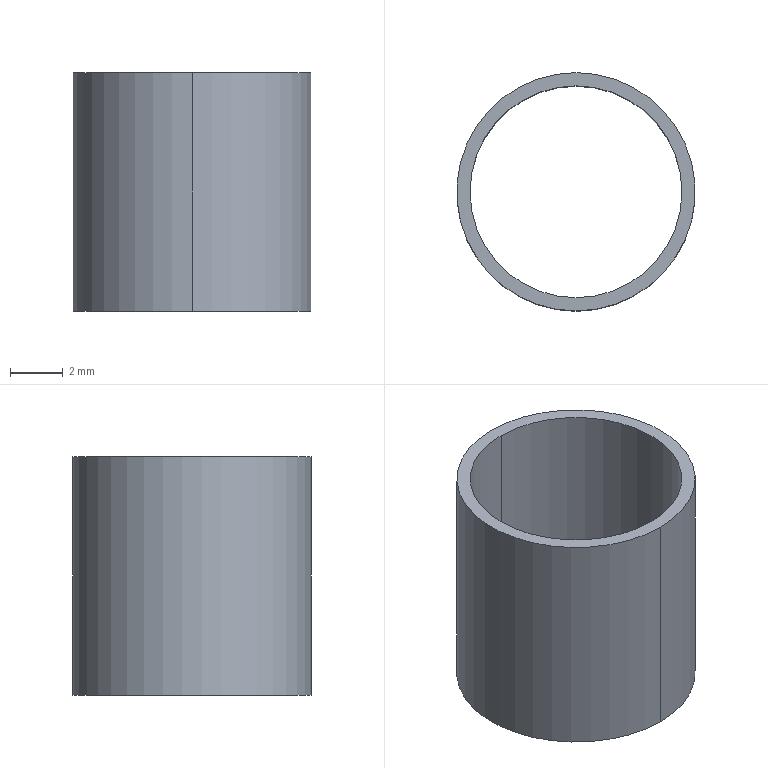Part | STEP file | ASND-0110-4216111700 | 1 solid | 6 faces | box 9 x 9 x 9 mm | volume 120.166 mm3 | cylinder 4 | plane 2 | commonest cylinder face diameters 8 x2 9 x2
STEP:
#1=CARTESIAN_POINT('',(0.,0.,0.));
#2=DIRECTION('',(0.,0.,1.));
#3=DIRECTION('',(1.,0.,0.));
#4=AXIS2_PLACEMENT_3D('',#1,#2,#3);
#5=CARTESIAN_POINT('',(0.,-4.,9.));
#6=VERTEX_POINT('',#5);
#7=CARTESIAN_POINT('',(0.,-4.,0.));
#8=VERTEX_POINT('',#7);
#9=CARTESIAN_POINT('',(0.,-4.,9.45));
#10=DIRECTION('',(0.,0.,-1.));
#11=VECTOR('',#10,1.);
#12=LINE('',#9,#11);
#13=CARTESIAN_POINT('',(0.,0.,9.45));
#14=DIRECTION('',(0.,0.,-1.));
#15=DIRECTION('',(0.,-1.,0.));
#16=AXIS2_PLACEMENT_3D('',#13,#14,#15);
#17=CYLINDRICAL_SURFACE('',#16,4.);
#18=CARTESIAN_POINT('',(6.283,0.));
#19=DIRECTION('',(0.,1.));
#20=VECTOR('',#19,1.);
#21=LINE('',#18,#20);
#22=(GEOMETRIC_REPRESENTATION_CONTEXT(2)PARAMETRIC_REPRESENTATION_CONTEXT()REPRESENTATION_CONTEXT('',''));
#23=DEFINITIONAL_REPRESENTATION('',(#21),#22);
#24=PCURVE('',#17,#23);
#25=CARTESIAN_POINT('',(0.,0.,9.45));
#26=DIRECTION('',(0.,0.,-1.));
#27=DIRECTION('',(0.,-1.,0.));
#28=AXIS2_PLACEMENT_3D('',#25,#26,#27);
#29=CYLINDRICAL_SURFACE('',#28,4.);
#30=CARTESIAN_POINT('',(0.,0.));
#31=DIRECTION('',(0.,1.));
#32=VECTOR('',#31,1.);
#33=LINE('',#30,#32);
#34=(GEOMETRIC_REPRESENTATION_CONTEXT(2)PARAMETRIC_REPRESENTATION_CONTEXT()REPRESENTATION_CONTEXT('',''));
#35=DEFINITIONAL_REPRESENTATION('',(#33),#34);
#36=PCURVE('',#29,#35);
#37=SURFACE_CURVE('',#12,(#24,#36),.PCURVE_S1.);
#38=EDGE_CURVE('',#6,#8,#37,.T.);
#39=ORIENTED_EDGE('',*,*,#38,.T.);
#40=CARTESIAN_POINT('',(0.,4.,0.));
#41=VERTEX_POINT('',#40);
#42=CARTESIAN_POINT('',(0.,0.,0.));
#43=DIRECTION('',(0.,0.,-1.));
#44=DIRECTION('',(0.,1.,0.));
#45=AXIS2_PLACEMENT_3D('',#42,#43,#44);
#46=CIRCLE('',#45,4.);
#47=CARTESIAN_POINT('',(3.142,9.45));
#48=DIRECTION('',(1.,0.));
#49=VECTOR('',#48,1.);
#50=LINE('',#47,#49);
#51=(GEOMETRIC_REPRESENTATION_CONTEXT(2)PARAMETRIC_REPRESENTATION_CONTEXT()REPRESENTATION_CONTEXT('',''));
#52=DEFINITIONAL_REPRESENTATION('',(#50),#51);
#53=PCURVE('',#17,#52);
#54=CARTESIAN_POINT('',(0.,0.,0.));
#55=DIRECTION('',(0.,0.,-1.));
#56=DIRECTION('',(0.7071,0.7071,0.));
#57=AXIS2_PLACEMENT_3D('',#54,#55,#56);
#58=PLANE('',#57);
#59=CARTESIAN_POINT('',(0.,0.));
#60=DIRECTION('',(0.7071,-0.7071));
#61=AXIS2_PLACEMENT_2D('',#59,#60);
#62=CIRCLE('',#61,4.);
#63=(GEOMETRIC_REPRESENTATION_CONTEXT(2)PARAMETRIC_REPRESENTATION_CONTEXT()REPRESENTATION_CONTEXT('',''));
#64=DEFINITIONAL_REPRESENTATION('',(#62),#63);
#65=PCURVE('',#58,#64);
#66=SURFACE_CURVE('',#46,(#53,#65),.PCURVE_S1.);
#67=EDGE_CURVE('',#41,#8,#66,.T.);
#68=ORIENTED_EDGE('',*,*,#67,.F.);
#69=CARTESIAN_POINT('',(0.,4.,9.));
#70=VERTEX_POINT('',#69);
#71=CARTESIAN_POINT('',(0.,4.,9.45));
#72=DIRECTION('',(0.,0.,-1.));
#73=VECTOR('',#72,1.);
#74=LINE('',#71,#73);
#75=CARTESIAN_POINT('',(3.142,0.));
#76=DIRECTION('',(0.,1.));
#77=VECTOR('',#76,1.);
#78=LINE('',#75,#77);
#79=(GEOMETRIC_REPRESENTATION_CONTEXT(2)PARAMETRIC_REPRESENTATION_CONTEXT()REPRESENTATION_CONTEXT('',''));
#80=DEFINITIONAL_REPRESENTATION('',(#78),#79);
#81=PCURVE('',#17,#80);
#82=CARTESIAN_POINT('',(3.142,0.));
#83=DIRECTION('',(0.,1.));
#84=VECTOR('',#83,1.);
#85=LINE('',#82,#84);
#86=(GEOMETRIC_REPRESENTATION_CONTEXT(2)PARAMETRIC_REPRESENTATION_CONTEXT()REPRESENTATION_CONTEXT('',''));
#87=DEFINITIONAL_REPRESENTATION('',(#85),#86);
#88=PCURVE('',#29,#87);
#89=SURFACE_CURVE('',#74,(#81,#88),.PCURVE_S1.);
#90=EDGE_CURVE('',#70,#41,#89,.T.);
#91=ORIENTED_EDGE('',*,*,#90,.F.);
#92=CARTESIAN_POINT('',(0.,0.,9.));
#93=DIRECTION('',(0.,0.,-1.));
#94=DIRECTION('',(0.,1.,0.));
#95=AXIS2_PLACEMENT_3D('',#92,#93,#94);
#96=CIRCLE('',#95,4.);
#97=CARTESIAN_POINT('',(3.142,0.45));
#98=DIRECTION('',(1.,0.));
#99=VECTOR('',#98,1.);
#100=LINE('',#97,#99);
#101=(GEOMETRIC_REPRESENTATION_CONTEXT(2)PARAMETRIC_REPRESENTATION_CONTEXT()REPRESENTATION_CONTEXT('',''));
#102=DEFINITIONAL_REPRESENTATION('',(#100),#101);
#103=PCURVE('',#17,#102);
#104=CARTESIAN_POINT('',(0.,0.,9.));
#105=DIRECTION('',(0.,0.,-1.));
#106=DIRECTION('',(0.7071,0.7071,0.));
#107=AXIS2_PLACEMENT_3D('',#104,#105,#106);
#108=PLANE('',#107);
#109=CARTESIAN_POINT('',(0.,0.));
#110=DIRECTION('',(0.7071,-0.7071));
#111=AXIS2_PLACEMENT_2D('',#109,#110);
#112=CIRCLE('',#111,4.);
#113=(GEOMETRIC_REPRESENTATION_CONTEXT(2)PARAMETRIC_REPRESENTATION_CONTEXT()REPRESENTATION_CONTEXT('',''));
#114=DEFINITIONAL_REPRESENTATION('',(#112),#113);
#115=PCURVE('',#108,#114);
#116=SURFACE_CURVE('',#96,(#103,#115),.PCURVE_S1.);
#117=EDGE_CURVE('',#70,#6,#116,.T.);
#118=ORIENTED_EDGE('',*,*,#117,.T.);
#119=EDGE_LOOP('',(#39,#68,#91,#118));
#120=FACE_BOUND('',#119,.F.);
#121=ADVANCED_FACE('',(#120),#17,.F.);
#122=CARTESIAN_POINT('',(0.,-4.5,9.));
#123=VERTEX_POINT('',#122);
#124=CARTESIAN_POINT('',(0.,4.5,9.));
#125=VERTEX_POINT('',#124);
#126=CARTESIAN_POINT('',(0.,0.,9.));
#127=DIRECTION('',(0.,0.,-1.));
#128=DIRECTION('',(0.,1.,0.));
#129=AXIS2_PLACEMENT_3D('',#126,#127,#128);
#130=CIRCLE('',#129,4.5);
#131=CARTESIAN_POINT('',(0.,0.,9.45));
#132=DIRECTION('',(0.,0.,-1.));
#133=DIRECTION('',(0.,-1.,0.));
#134=AXIS2_PLACEMENT_3D('',#131,#132,#133);
#135=CYLINDRICAL_SURFACE('',#134,4.5);
#136=CARTESIAN_POINT('',(-3.142,0.45));
#137=DIRECTION('',(1.,0.));
#138=VECTOR('',#137,1.);
#139=LINE('',#136,#138);
#140=(GEOMETRIC_REPRESENTATION_CONTEXT(2)PARAMETRIC_REPRESENTATION_CONTEXT()REPRESENTATION_CONTEXT('',''));
#141=DEFINITIONAL_REPRESENTATION('',(#139),#140);
#142=PCURVE('',#135,#141);
#143=CARTESIAN_POINT('',(0.,0.));
#144=DIRECTION('',(0.7071,-0.7071));
#145=AXIS2_PLACEMENT_2D('',#143,#144);
#146=CIRCLE('',#145,4.5);
#147=(GEOMETRIC_REPRESENTATION_CONTEXT(2)PARAMETRIC_REPRESENTATION_CONTEXT()REPRESENTATION_CONTEXT('',''));
#148=DEFINITIONAL_REPRESENTATION('',(#146),#147);
#149=PCURVE('',#108,#148);
#150=SURFACE_CURVE('',#130,(#142,#149),.PCURVE_S1.);
#151=EDGE_CURVE('',#123,#125,#150,.T.);
#152=ORIENTED_EDGE('',*,*,#151,.T.);
#153=CARTESIAN_POINT('',(0.,4.5,0.));
#154=VERTEX_POINT('',#153);
#155=CARTESIAN_POINT('',(0.,4.5,9.45));
#156=DIRECTION('',(0.,0.,-1.));
#157=VECTOR('',#156,1.);
#158=LINE('',#155,#157);
#159=CARTESIAN_POINT('',(3.142,0.));
#160=DIRECTION('',(0.,1.));
#161=VECTOR('',#160,1.);
#162=LINE('',#159,#161);
#163=(GEOMETRIC_REPRESENTATION_CONTEXT(2)PARAMETRIC_REPRESENTATION_CONTEXT()REPRESENTATION_CONTEXT('',''));
#164=DEFINITIONAL_REPRESENTATION('',(#162),#163);
#165=PCURVE('',#135,#164);
#166=CARTESIAN_POINT('',(0.,0.,9.45));
#167=DIRECTION('',(0.,0.,-1.));
#168=DIRECTION('',(0.,-1.,0.));
#169=AXIS2_PLACEMENT_3D('',#166,#167,#168);
#170=CYLINDRICAL_SURFACE('',#169,4.5);
#171=CARTESIAN_POINT('',(3.142,0.));
#172=DIRECTION('',(0.,1.));
#173=VECTOR('',#172,1.);
#174=LINE('',#171,#173);
#175=(GEOMETRIC_REPRESENTATION_CONTEXT(2)PARAMETRIC_REPRESENTATION_CONTEXT()REPRESENTATION_CONTEXT('',''));
#176=DEFINITIONAL_REPRESENTATION('',(#174),#175);
#177=PCURVE('',#170,#176);
#178=SURFACE_CURVE('',#158,(#165,#177),.PCURVE_S1.);
#179=EDGE_CURVE('',#125,#154,#178,.T.);
#180=ORIENTED_EDGE('',*,*,#179,.T.);
#181=CARTESIAN_POINT('',(0.,-4.5,0.));
#182=VERTEX_POINT('',#181);
#183=CARTESIAN_POINT('',(0.,0.,0.));
#184=DIRECTION('',(0.,0.,1.));
#185=DIRECTION('',(0.,1.,0.));
#186=AXIS2_PLACEMENT_3D('',#183,#184,#185);
#187=CIRCLE('',#186,4.5);
#188=CARTESIAN_POINT('',(3.142,9.45));
#189=DIRECTION('',(-1.,0.));
#190=VECTOR('',#189,1.);
#191=LINE('',#188,#190);
#192=(GEOMETRIC_REPRESENTATION_CONTEXT(2)PARAMETRIC_REPRESENTATION_CONTEXT()REPRESENTATION_CONTEXT('',''));
#193=DEFINITIONAL_REPRESENTATION('',(#191),#192);
#194=PCURVE('',#135,#193);
#195=CARTESIAN_POINT('',(3.182,-3.182));
#196=CARTESIAN_POINT('',(-2.329,-8.693));
#197=CARTESIAN_POINT('',(-4.347,-1.165));
#198=CARTESIAN_POINT('',(-6.364,6.364));
#199=CARTESIAN_POINT('',(1.165,4.347));
#200=CARTESIAN_POINT('',(8.693,2.329));
#201=CARTESIAN_POINT('',(3.182,-3.182));
#202=(BOUNDED_CURVE()B_SPLINE_CURVE(2,(#195,#196,#197,#198,#199,#200,#201),.UNSPECIFIED.,.T.,.F.)B_SPLINE_CURVE_WITH_KNOTS((1,2,2,2,2,1),(-2.094,0.,2.094,4.189,6.283,8.378),.UNSPECIFIED.)CURVE()GEOMETRIC_REPRESENTATION_ITEM()RATIONAL_B_SPLINE_CURVE((1.,0.5,1.,0.5,1.,0.5,1.))REPRESENTATION_ITEM(''));
#203=(GEOMETRIC_REPRESENTATION_CONTEXT(2)PARAMETRIC_REPRESENTATION_CONTEXT()REPRESENTATION_CONTEXT('',''));
#204=DEFINITIONAL_REPRESENTATION('',(#202),#203);
#205=PCURVE('',#58,#204);
#206=SURFACE_CURVE('',#187,(#194,#205),.PCURVE_S1.);
#207=EDGE_CURVE('',#154,#182,#206,.T.);
#208=ORIENTED_EDGE('',*,*,#207,.T.);
#209=CARTESIAN_POINT('',(0.,-4.5,9.45));
#210=DIRECTION('',(0.,0.,-1.));
#211=VECTOR('',#210,1.);
#212=LINE('',#209,#211);
#213=CARTESIAN_POINT('',(0.,0.));
#214=DIRECTION('',(0.,1.));
#215=VECTOR('',#214,1.);
#216=LINE('',#213,#215);
#217=(GEOMETRIC_REPRESENTATION_CONTEXT(2)PARAMETRIC_REPRESENTATION_CONTEXT()REPRESENTATION_CONTEXT('',''));
#218=DEFINITIONAL_REPRESENTATION('',(#216),#217);
#219=PCURVE('',#135,#218);
#220=CARTESIAN_POINT('',(6.283,0.));
#221=DIRECTION('',(0.,1.));
#222=VECTOR('',#221,1.);
#223=LINE('',#220,#222);
#224=(GEOMETRIC_REPRESENTATION_CONTEXT(2)PARAMETRIC_REPRESENTATION_CONTEXT()REPRESENTATION_CONTEXT('',''));
#225=DEFINITIONAL_REPRESENTATION('',(#223),#224);
#226=PCURVE('',#170,#225);
#227=SURFACE_CURVE('',#212,(#219,#226),.PCURVE_S1.);
#228=EDGE_CURVE('',#123,#182,#227,.T.);
#229=ORIENTED_EDGE('',*,*,#228,.F.);
#230=EDGE_LOOP('',(#152,#180,#208,#229));
#231=FACE_BOUND('',#230,.T.);
#232=ADVANCED_FACE('',(#231),#135,.T.);
#233=ORIENTED_EDGE('',*,*,#179,.F.);
#234=CARTESIAN_POINT('',(0.,0.,9.));
#235=DIRECTION('',(0.,0.,-1.));
#236=DIRECTION('',(0.,1.,0.));
#237=AXIS2_PLACEMENT_3D('',#234,#235,#236);
#238=CIRCLE('',#237,4.5);
#239=CARTESIAN_POINT('',(3.142,0.45));
#240=DIRECTION('',(1.,0.));
#241=VECTOR('',#240,1.);
#242=LINE('',#239,#241);
#243=(GEOMETRIC_REPRESENTATION_CONTEXT(2)PARAMETRIC_REPRESENTATION_CONTEXT()REPRESENTATION_CONTEXT('',''));
#244=DEFINITIONAL_REPRESENTATION('',(#242),#243);
#245=PCURVE('',#170,#244);
#246=CARTESIAN_POINT('',(0.,0.));
#247=DIRECTION('',(0.7071,-0.7071));
#248=AXIS2_PLACEMENT_2D('',#246,#247);
#249=CIRCLE('',#248,4.5);
#250=(GEOMETRIC_REPRESENTATION_CONTEXT(2)PARAMETRIC_REPRESENTATION_CONTEXT()REPRESENTATION_CONTEXT('',''));
#251=DEFINITIONAL_REPRESENTATION('',(#249),#250);
#252=PCURVE('',#108,#251);
#253=SURFACE_CURVE('',#238,(#245,#252),.PCURVE_S1.);
#254=EDGE_CURVE('',#125,#123,#253,.T.);
#255=ORIENTED_EDGE('',*,*,#254,.T.);
#256=ORIENTED_EDGE('',*,*,#228,.T.);
#257=CARTESIAN_POINT('',(0.,0.,0.));
#258=DIRECTION('',(0.,0.,1.));
#259=DIRECTION('',(0.,1.,0.));
#260=AXIS2_PLACEMENT_3D('',#257,#258,#259);
#261=CIRCLE('',#260,4.5);
#262=CARTESIAN_POINT('',(9.425,9.45));
#263=DIRECTION('',(-1.,0.));
#264=VECTOR('',#263,1.);
#265=LINE('',#262,#264);
#266=(GEOMETRIC_REPRESENTATION_CONTEXT(2)PARAMETRIC_REPRESENTATION_CONTEXT()REPRESENTATION_CONTEXT('',''));
#267=DEFINITIONAL_REPRESENTATION('',(#265),#266);
#268=PCURVE('',#170,#267);
#269=CARTESIAN_POINT('',(3.182,-3.182));
#270=CARTESIAN_POINT('',(-2.329,-8.693));
#271=CARTESIAN_POINT('',(-4.347,-1.165));
#272=CARTESIAN_POINT('',(-6.364,6.364));
#273=CARTESIAN_POINT('',(1.165,4.347));
#274=CARTESIAN_POINT('',(8.693,2.329));
#275=CARTESIAN_POINT('',(3.182,-3.182));
#276=(BOUNDED_CURVE()B_SPLINE_CURVE(2,(#269,#270,#271,#272,#273,#274,#275),.UNSPECIFIED.,.T.,.F.)B_SPLINE_CURVE_WITH_KNOTS((1,2,2,2,2,1),(-2.094,0.,2.094,4.189,6.283,8.378),.UNSPECIFIED.)CURVE()GEOMETRIC_REPRESENTATION_ITEM()RATIONAL_B_SPLINE_CURVE((1.,0.5,1.,0.5,1.,0.5,1.))REPRESENTATION_ITEM(''));
#277=(GEOMETRIC_REPRESENTATION_CONTEXT(2)PARAMETRIC_REPRESENTATION_CONTEXT()REPRESENTATION_CONTEXT('',''));
#278=DEFINITIONAL_REPRESENTATION('',(#276),#277);
#279=PCURVE('',#58,#278);
#280=SURFACE_CURVE('',#261,(#268,#279),.PCURVE_S1.);
#281=EDGE_CURVE('',#182,#154,#280,.T.);
#282=ORIENTED_EDGE('',*,*,#281,.T.);
#283=EDGE_LOOP('',(#233,#255,#256,#282));
#284=FACE_BOUND('',#283,.T.);
#285=ADVANCED_FACE('',(#284),#170,.T.);
#286=ORIENTED_EDGE('',*,*,#151,.F.);
#287=ORIENTED_EDGE('',*,*,#254,.F.);
#288=EDGE_LOOP('',(#286,#287));
#289=FACE_BOUND('',#288,.T.);
#290=CARTESIAN_POINT('',(0.,0.,9.));
#291=DIRECTION('',(0.,0.,-1.));
#292=DIRECTION('',(0.,1.,0.));
#293=AXIS2_PLACEMENT_3D('',#290,#291,#292);
#294=CIRCLE('',#293,4.);
#295=CARTESIAN_POINT('',(0.,0.));
#296=DIRECTION('',(0.7071,-0.7071));
#297=AXIS2_PLACEMENT_2D('',#295,#296);
#298=CIRCLE('',#297,4.);
#299=(GEOMETRIC_REPRESENTATION_CONTEXT(2)PARAMETRIC_REPRESENTATION_CONTEXT()REPRESENTATION_CONTEXT('',''));
#300=DEFINITIONAL_REPRESENTATION('',(#298),#299);
#301=PCURVE('',#108,#300);
#302=CARTESIAN_POINT('',(-3.142,0.45));
#303=DIRECTION('',(1.,0.));
#304=VECTOR('',#303,1.);
#305=LINE('',#302,#304);
#306=(GEOMETRIC_REPRESENTATION_CONTEXT(2)PARAMETRIC_REPRESENTATION_CONTEXT()REPRESENTATION_CONTEXT('',''));
#307=DEFINITIONAL_REPRESENTATION('',(#305),#306);
#308=PCURVE('',#29,#307);
#309=SURFACE_CURVE('',#294,(#301,#308),.PCURVE_S1.);
#310=EDGE_CURVE('',#6,#70,#309,.T.);
#311=ORIENTED_EDGE('',*,*,#310,.T.);
#312=ORIENTED_EDGE('',*,*,#117,.T.);
#313=EDGE_LOOP('',(#311,#312));
#314=FACE_BOUND('',#313,.T.);
#315=ADVANCED_FACE('',(#289,#314),#108,.F.);
#316=CARTESIAN_POINT('',(0.,0.,0.));
#317=DIRECTION('',(0.,0.,-1.));
#318=DIRECTION('',(0.,1.,0.));
#319=AXIS2_PLACEMENT_3D('',#316,#317,#318);
#320=CIRCLE('',#319,4.);
#321=CARTESIAN_POINT('',(-3.142,9.45));
#322=DIRECTION('',(1.,0.));
#323=VECTOR('',#322,1.);
#324=LINE('',#321,#323);
#325=(GEOMETRIC_REPRESENTATION_CONTEXT(2)PARAMETRIC_REPRESENTATION_CONTEXT()REPRESENTATION_CONTEXT('',''));
#326=DEFINITIONAL_REPRESENTATION('',(#324),#325);
#327=PCURVE('',#29,#326);
#328=CARTESIAN_POINT('',(0.,0.));
#329=DIRECTION('',(0.7071,-0.7071));
#330=AXIS2_PLACEMENT_2D('',#328,#329);
#331=CIRCLE('',#330,4.);
#332=(GEOMETRIC_REPRESENTATION_CONTEXT(2)PARAMETRIC_REPRESENTATION_CONTEXT()REPRESENTATION_CONTEXT('',''));
#333=DEFINITIONAL_REPRESENTATION('',(#331),#332);
#334=PCURVE('',#58,#333);
#335=SURFACE_CURVE('',#320,(#327,#334),.PCURVE_S1.);
#336=EDGE_CURVE('',#8,#41,#335,.T.);
#337=ORIENTED_EDGE('',*,*,#336,.F.);
#338=ORIENTED_EDGE('',*,*,#38,.F.);
#339=ORIENTED_EDGE('',*,*,#310,.T.);
#340=ORIENTED_EDGE('',*,*,#90,.T.);
#341=EDGE_LOOP('',(#337,#338,#339,#340));
#342=FACE_BOUND('',#341,.F.);
#343=ADVANCED_FACE('',(#342),#29,.F.);
#344=ORIENTED_EDGE('',*,*,#281,.F.);
#345=ORIENTED_EDGE('',*,*,#207,.F.);
#346=EDGE_LOOP('',(#344,#345));
#347=FACE_BOUND('',#346,.T.);
#348=ORIENTED_EDGE('',*,*,#336,.F.);
#349=ORIENTED_EDGE('',*,*,#67,.F.);
#350=EDGE_LOOP('',(#348,#349));
#351=FACE_BOUND('',#350,.T.);
#352=ADVANCED_FACE('',(#347,#351),#58,.T.);
#353=CLOSED_SHELL('',(#121,#232,#285,#315,#343,#352));
#354=MANIFOLD_SOLID_BREP('',#353);
#355=(LENGTH_UNIT()NAMED_UNIT(*)SI_UNIT(.MILLI.,.METRE.));
#356=UNCERTAINTY_MEASURE_WITH_UNIT(LENGTH_MEASURE(0.0000001),#355,'','');
#357=(NAMED_UNIT(*)PLANE_ANGLE_UNIT()SI_UNIT($,.RADIAN.));
#358=(NAMED_UNIT(*)SI_UNIT($,.STERADIAN.)SOLID_ANGLE_UNIT());
#359=(GEOMETRIC_REPRESENTATION_CONTEXT(3)GLOBAL_UNCERTAINTY_ASSIGNED_CONTEXT((#356))GLOBAL_UNIT_ASSIGNED_CONTEXT((#355,#357,#358))REPRESENTATION_CONTEXT('',''));
#360=ADVANCED_BREP_SHAPE_REPRESENTATION('',(#4,#354),#359);